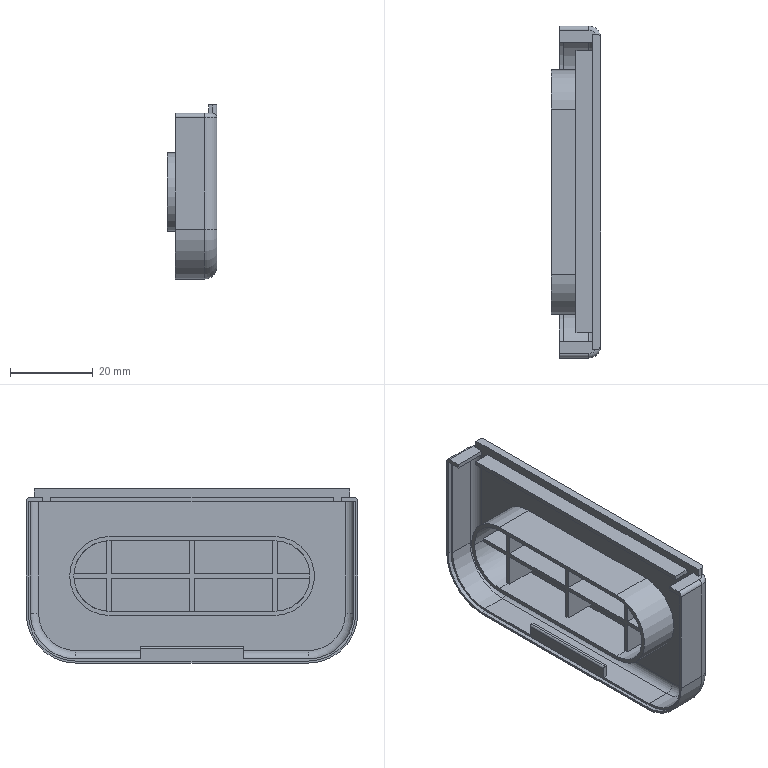Part | SolidWorks | features BossThin 5, Fillet 4, ICE 3, FillRefSurface 1, SewRefSurface 1, Shell 1, Stock 1, SurfCut 1, SweepCut 1, TrimRefSurface 1 | 1 solid | 94 faces | box 12 x 80 x 42 mm | volume 7212 mm3 | plane 65 | cylinder 23 | torus 6 | commonest cylinder face diameters 2 x4 4 x3 6 x3 17 x3 19 x3 22 x2